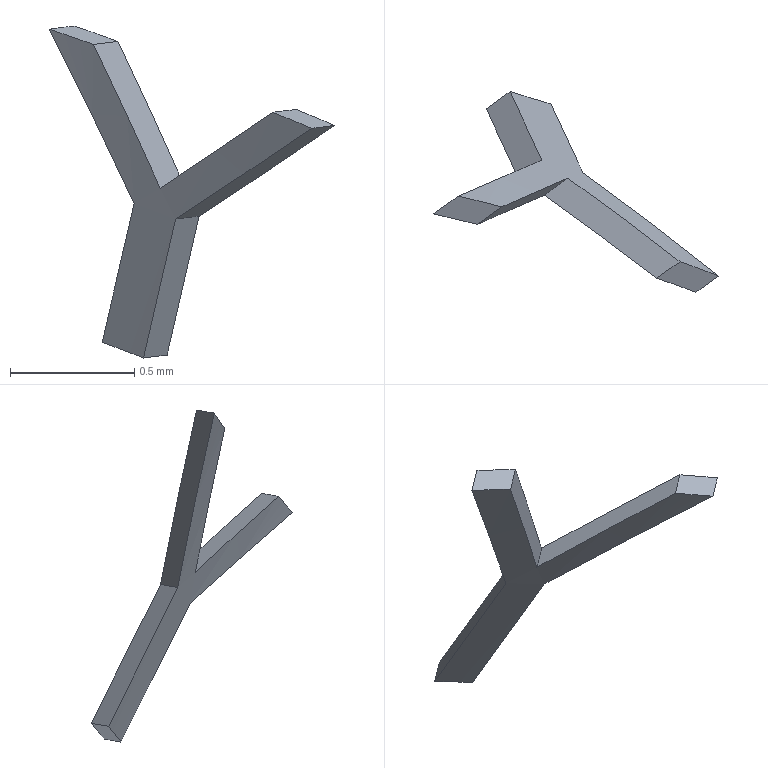Part | SolidWorks | features BaseBody 1 | 1 solid | 11 faces | box 1.15 x 0.8105 x 1.338 mm | volume 0.03304 mm3 | plane 9 | cylinder 2 | commonest cylinder face diameters 16.8 x1 17 x1
STEP:
#1=CARTESIAN_POINT('',(1969.96,-236.727,996.491));
#2=VERTEX_POINT('',#1);
#3=CARTESIAN_POINT('',(1970.089,-237.005,997.05));
#4=VERTEX_POINT('',#3);
#5=CARTESIAN_POINT('',(1970.77,-238.48,1000.016));
#6=DIRECTION('',(0.2015,-0.436,0.8771));
#7=VECTOR('',#6,1000.);
#8=LINE('',#5,#7);
#9=EDGE_CURVE('',#2,#4,#8,.T.);
#10=ORIENTED_EDGE('',*,*,#9,.T.);
#11=CARTESIAN_POINT('',(1970.638,-237.419,997.416));
#12=VERTEX_POINT('',#11);
#13=CARTESIAN_POINT('',(1970.089,-237.005,997.05));
#14=CARTESIAN_POINT('',(1970.275,-237.139,997.172));
#15=CARTESIAN_POINT('',(1970.458,-237.277,997.294));
#16=CARTESIAN_POINT('',(1970.638,-237.419,997.416));
#17=B_SPLINE_CURVE_WITH_KNOTS('',3,(#13,#14,#15,#16),.UNSPECIFIED.,.F.,.F.,(4,4),(0.,1.),.UNSPECIFIED.);
#18=EDGE_CURVE('',#4,#12,#17,.T.);
#19=ORIENTED_EDGE('',*,*,#18,.T.);
#20=CARTESIAN_POINT('',(1970.482,-237.362,997.481));
#21=VERTEX_POINT('',#20);
#22=CARTESIAN_POINT('',(1966.892,-244.458,994.777));
#23=DIRECTION('',(0.2015,-0.436,0.8771));
#24=DIRECTION('',(-0.7309,-0.6631,-0.1618));
#25=AXIS2_PLACEMENT_3D('',#22,#23,#24);
#26=CIRCLE('',#25,8.4);
#27=EDGE_CURVE('',#12,#21,#26,.T.);
#28=ORIENTED_EDGE('',*,*,#27,.T.);
#29=CARTESIAN_POINT('',(1970.027,-237.026,997.175));
#30=VERTEX_POINT('',#29);
#31=CARTESIAN_POINT('',(1970.027,-237.026,997.175));
#32=CARTESIAN_POINT('',(1970.181,-237.135,997.277));
#33=CARTESIAN_POINT('',(1970.332,-237.247,997.379));
#34=CARTESIAN_POINT('',(1970.482,-237.362,997.481));
#35=B_SPLINE_CURVE_WITH_KNOTS('',3,(#31,#32,#33,#34),.UNSPECIFIED.,.F.,.F.,(4,4),(0.,1.),.UNSPECIFIED.);
#36=EDGE_CURVE('',#30,#21,#35,.T.);
#37=ORIENTED_EDGE('',*,*,#36,.F.);
#38=CARTESIAN_POINT('',(1969.758,-237.145,997.754));
#39=VERTEX_POINT('',#38);
#40=CARTESIAN_POINT('',(1969.758,-237.145,997.754));
#41=CARTESIAN_POINT('',(1969.85,-237.104,997.563));
#42=CARTESIAN_POINT('',(1969.94,-237.064,997.37));
#43=CARTESIAN_POINT('',(1970.027,-237.026,997.175));
#44=B_SPLINE_CURVE_WITH_KNOTS('',3,(#40,#41,#42,#43),.UNSPECIFIED.,.F.,.F.,(4,4),(0.,1.),.UNSPECIFIED.);
#45=EDGE_CURVE('',#39,#30,#44,.T.);
#46=ORIENTED_EDGE('',*,*,#45,.F.);
#47=CARTESIAN_POINT('',(1969.58,-237.103,997.816));
#48=VERTEX_POINT('',#47);
#49=CARTESIAN_POINT('',(1966.892,-244.458,994.777));
#50=DIRECTION('',(0.2015,-0.436,0.8771));
#51=DIRECTION('',(-0.7309,-0.6631,-0.1618));
#52=AXIS2_PLACEMENT_3D('',#49,#50,#51);
#53=CIRCLE('',#52,8.4);
#54=EDGE_CURVE('',#39,#48,#53,.T.);
#55=ORIENTED_EDGE('',*,*,#54,.T.);
#56=CARTESIAN_POINT('',(1969.922,-236.955,997.114));
#57=VERTEX_POINT('',#56);
#58=CARTESIAN_POINT('',(1969.58,-237.103,997.816));
#59=CARTESIAN_POINT('',(1969.698,-237.051,997.585));
#60=CARTESIAN_POINT('',(1969.812,-237.002,997.35));
#61=CARTESIAN_POINT('',(1969.922,-236.955,997.114));
#62=B_SPLINE_CURVE_WITH_KNOTS('',3,(#58,#59,#60,#61),.UNSPECIFIED.,.F.,.F.,(4,4),(0.,1.),.UNSPECIFIED.);
#63=EDGE_CURVE('',#48,#57,#62,.T.);
#64=ORIENTED_EDGE('',*,*,#63,.T.);
#65=CARTESIAN_POINT('',(1969.793,-236.677,996.554));
#66=VERTEX_POINT('',#65);
#67=CARTESIAN_POINT('',(1970.603,-238.43,1000.08));
#68=DIRECTION('',(-0.2015,0.436,-0.8771));
#69=VECTOR('',#68,1000.);
#70=LINE('',#67,#69);
#71=EDGE_CURVE('',#57,#66,#70,.T.);
#72=ORIENTED_EDGE('',*,*,#71,.T.);
#73=CARTESIAN_POINT('',(1966.64,-243.913,993.681));
#74=DIRECTION('',(-0.2015,0.436,-0.8771));
#75=DIRECTION('',(-0.7309,-0.6631,-0.1618));
#76=AXIS2_PLACEMENT_3D('',#73,#74,#75);
#77=CIRCLE('',#76,8.4);
#78=EDGE_CURVE('',#66,#2,#77,.T.);
#79=ORIENTED_EDGE('',*,*,#78,.T.);
#80=EDGE_LOOP('',(#10,#19,#28,#37,#46,#55,#64,#72,#79));
#81=FACE_OUTER_BOUND('',#80,.T.);
#82=CARTESIAN_POINT('',(1967.45,-245.666,997.207));
#83=DIRECTION('',(0.2015,-0.436,0.8771));
#84=DIRECTION('',(-0.7309,-0.6631,-0.1618));
#85=AXIS2_PLACEMENT_3D('',#82,#83,#84);
#86=CYLINDRICAL_SURFACE('',#85,8.4);
#87=ADVANCED_FACE('',(#81),#86,.F.);
#88=CARTESIAN_POINT('',(1970.055,-236.659,996.503));
#89=VERTEX_POINT('',#88);
#90=CARTESIAN_POINT('',(1970.008,-236.693,996.497));
#91=DIRECTION('',(-0.8088,-0.5792,-0.1022));
#92=VECTOR('',#91,1000.);
#93=LINE('',#90,#92);
#94=EDGE_CURVE('',#89,#2,#93,.T.);
#95=ORIENTED_EDGE('',*,*,#94,.T.);
#96=ORIENTED_EDGE('',*,*,#78,.F.);
#97=CARTESIAN_POINT('',(1969.89,-236.608,996.566));
#98=VERTEX_POINT('',#97);
#99=CARTESIAN_POINT('',(1969.841,-236.643,996.56));
#100=DIRECTION('',(-0.8088,-0.5792,-0.1022));
#101=VECTOR('',#100,1000.);
#102=LINE('',#99,#101);
#103=EDGE_CURVE('',#98,#66,#102,.T.);
#104=ORIENTED_EDGE('',*,*,#103,.F.);
#105=CARTESIAN_POINT('',(1966.64,-243.913,993.681));
#106=DIRECTION('',(-0.2015,0.436,-0.8771));
#107=DIRECTION('',(-0.7309,-0.6631,-0.1618));
#108=AXIS2_PLACEMENT_3D('',#105,#106,#107);
#109=CIRCLE('',#108,8.5);
#110=EDGE_CURVE('',#98,#89,#109,.T.);
#111=ORIENTED_EDGE('',*,*,#110,.T.);
#112=EDGE_LOOP('',(#95,#96,#104,#111));
#113=FACE_OUTER_BOUND('',#112,.T.);
#114=CARTESIAN_POINT('',(1982.308,-239.633,992.21));
#115=DIRECTION('',(-0.2015,0.436,-0.8771));
#116=DIRECTION('',(-0.5526,0.6888,0.4693));
#117=AXIS2_PLACEMENT_3D('',#114,#115,#116);
#118=PLANE('',#117);
#119=ADVANCED_FACE('',(#113),#118,.T.);
#120=ORIENTED_EDGE('',*,*,#103,.T.);
#121=ORIENTED_EDGE('',*,*,#71,.F.);
#122=CARTESIAN_POINT('',(1970.018,-236.886,997.126));
#123=VERTEX_POINT('',#122);
#124=CARTESIAN_POINT('',(1969.97,-236.921,997.12));
#125=DIRECTION('',(-0.8088,-0.5792,-0.1022));
#126=VECTOR('',#125,1000.);
#127=LINE('',#124,#126);
#128=EDGE_CURVE('',#123,#57,#127,.T.);
#129=ORIENTED_EDGE('',*,*,#128,.F.);
#130=CARTESIAN_POINT('',(1969.954,-236.747,996.846));
#131=DIRECTION('',(-0.2015,0.436,-0.8771));
#132=VECTOR('',#131,1000.);
#133=LINE('',#130,#132);
#134=EDGE_CURVE('',#123,#98,#133,.T.);
#135=ORIENTED_EDGE('',*,*,#134,.T.);
#136=EDGE_LOOP('',(#120,#121,#129,#135));
#137=FACE_OUTER_BOUND('',#136,.T.);
#138=CARTESIAN_POINT('',(1976.364,-232.342,997.927));
#139=DIRECTION('',(-0.5526,0.6888,0.4693));
#140=DIRECTION('',(0.2015,-0.436,0.8771));
#141=AXIS2_PLACEMENT_3D('',#138,#139,#140);
#142=PLANE('',#141);
#143=ADVANCED_FACE('',(#137),#142,.T.);
#144=ORIENTED_EDGE('',*,*,#128,.T.);
#145=ORIENTED_EDGE('',*,*,#63,.F.);
#146=CARTESIAN_POINT('',(1969.681,-237.031,997.829));
#147=VERTEX_POINT('',#146);
#148=CARTESIAN_POINT('',(1969.63,-237.067,997.822));
#149=DIRECTION('',(-0.8088,-0.5792,-0.1022));
#150=VECTOR('',#149,1000.);
#151=LINE('',#148,#150);
#152=EDGE_CURVE('',#147,#48,#151,.T.);
#153=ORIENTED_EDGE('',*,*,#152,.F.);
#154=CARTESIAN_POINT('',(1969.681,-237.031,997.829));
#155=CARTESIAN_POINT('',(1969.751,-237.,997.69));
#156=CARTESIAN_POINT('',(1969.819,-236.971,997.55));
#157=CARTESIAN_POINT('',(1969.887,-236.942,997.409));
#158=CARTESIAN_POINT('',(1969.953,-236.914,997.268));
#159=CARTESIAN_POINT('',(1970.018,-236.886,997.126));
#160=B_SPLINE_CURVE_WITH_KNOTS('',5,(#154,#155,#156,#157,#158,#159),.UNSPECIFIED.,.F.,.F.,(6,6),(0.,1.),.UNSPECIFIED.);
#161=EDGE_CURVE('',#147,#123,#160,.T.);
#162=ORIENTED_EDGE('',*,*,#161,.T.);
#163=EDGE_LOOP('',(#144,#145,#153,#162));
#164=FACE_OUTER_BOUND('',#163,.T.);
#165=CARTESIAN_POINT('',(1976.257,-232.322,998.66));
#166=DIRECTION('',(-0.5701,0.8147,-0.1059));
#167=DIRECTION('',(-0.1446,0.02737,0.9891));
#168=AXIS2_PLACEMENT_3D('',#165,#166,#167);
#169=PLANE('',#168);
#170=ADVANCED_FACE('',(#164),#169,.T.);
#171=ORIENTED_EDGE('',*,*,#152,.T.);
#172=ORIENTED_EDGE('',*,*,#54,.F.);
#173=CARTESIAN_POINT('',(1969.857,-237.075,997.767));
#174=VERTEX_POINT('',#173);
#175=CARTESIAN_POINT('',(1969.807,-237.11,997.761));
#176=DIRECTION('',(-0.8088,-0.5792,-0.1022));
#177=VECTOR('',#176,1000.);
#178=LINE('',#175,#177);
#179=EDGE_CURVE('',#174,#39,#178,.T.);
#180=ORIENTED_EDGE('',*,*,#179,.F.);
#181=CARTESIAN_POINT('',(1966.892,-244.458,994.777));
#182=DIRECTION('',(0.2015,-0.436,0.8771));
#183=DIRECTION('',(-0.7309,-0.6631,-0.1618));
#184=AXIS2_PLACEMENT_3D('',#181,#182,#183);
#185=CIRCLE('',#184,8.5);
#186=EDGE_CURVE('',#174,#147,#185,.T.);
#187=ORIENTED_EDGE('',*,*,#186,.T.);
#188=EDGE_LOOP('',(#171,#172,#180,#187));
#189=FACE_OUTER_BOUND('',#188,.T.);
#190=CARTESIAN_POINT('',(1982.415,-239.999,993.428));
#191=DIRECTION('',(0.2015,-0.436,0.8771));
#192=DIRECTION('',(0.5526,-0.6888,-0.4693));
#193=AXIS2_PLACEMENT_3D('',#190,#191,#192);
#194=PLANE('',#193);
#195=ADVANCED_FACE('',(#189),#194,.T.);
#196=ORIENTED_EDGE('',*,*,#179,.T.);
#197=ORIENTED_EDGE('',*,*,#45,.T.);
#198=CARTESIAN_POINT('',(1970.123,-236.958,997.187));
#199=VERTEX_POINT('',#198);
#200=CARTESIAN_POINT('',(1970.075,-236.992,997.181));
#201=DIRECTION('',(-0.8088,-0.5792,-0.1022));
#202=VECTOR('',#201,1000.);
#203=LINE('',#200,#202);
#204=EDGE_CURVE('',#199,#30,#203,.T.);
#205=ORIENTED_EDGE('',*,*,#204,.F.);
#206=CARTESIAN_POINT('',(1969.857,-237.075,997.767));
#207=CARTESIAN_POINT('',(1969.912,-237.05,997.652));
#208=CARTESIAN_POINT('',(1969.966,-237.026,997.536));
#209=CARTESIAN_POINT('',(1970.019,-237.003,997.421));
#210=CARTESIAN_POINT('',(1970.071,-236.98,997.304));
#211=CARTESIAN_POINT('',(1970.123,-236.958,997.187));
#212=B_SPLINE_CURVE_WITH_KNOTS('',5,(#206,#207,#208,#209,#210,#211),.UNSPECIFIED.,.F.,.F.,(6,6),(0.,1.),.UNSPECIFIED.);
#213=EDGE_CURVE('',#174,#199,#212,.T.);
#214=ORIENTED_EDGE('',*,*,#213,.F.);
#215=EDGE_LOOP('',(#196,#197,#205,#214));
#216=FACE_OUTER_BOUND('',#215,.T.);
#217=CARTESIAN_POINT('',(1976.428,-232.442,997.984));
#218=DIRECTION('',(0.5712,-0.8149,0.09826));
#219=DIRECTION('',(0.1402,-0.0211,-0.9899));
#220=AXIS2_PLACEMENT_3D('',#217,#218,#219);
#221=PLANE('',#220);
#222=ADVANCED_FACE('',(#216),#221,.T.);
#223=ORIENTED_EDGE('',*,*,#204,.T.);
#224=ORIENTED_EDGE('',*,*,#36,.T.);
#225=CARTESIAN_POINT('',(1970.575,-237.295,997.492));
#226=VERTEX_POINT('',#225);
#227=CARTESIAN_POINT('',(1970.528,-237.328,997.486));
#228=DIRECTION('',(-0.8088,-0.5792,-0.1022));
#229=VECTOR('',#228,1000.);
#230=LINE('',#227,#229);
#231=EDGE_CURVE('',#226,#21,#230,.T.);
#232=ORIENTED_EDGE('',*,*,#231,.F.);
#233=CARTESIAN_POINT('',(1970.123,-236.958,997.187));
#234=CARTESIAN_POINT('',(1970.214,-237.024,997.248));
#235=CARTESIAN_POINT('',(1970.305,-237.09,997.309));
#236=CARTESIAN_POINT('',(1970.396,-237.158,997.37));
#237=CARTESIAN_POINT('',(1970.485,-237.226,997.431));
#238=CARTESIAN_POINT('',(1970.575,-237.295,997.492));
#239=B_SPLINE_CURVE_WITH_KNOTS('',5,(#233,#234,#235,#236,#237,#238),.UNSPECIFIED.,.F.,.F.,(6,6),(0.,1.),.UNSPECIFIED.);
#240=EDGE_CURVE('',#199,#226,#239,.T.);
#241=ORIENTED_EDGE('',*,*,#240,.F.);
#242=EDGE_LOOP('',(#223,#224,#232,#241));
#243=FACE_OUTER_BOUND('',#242,.T.);
#244=CARTESIAN_POINT('',(1976.717,-232.896,998.268));
#245=DIRECTION('',(-0.3469,0.3295,0.8781));
#246=DIRECTION('',(0.4749,-0.7456,0.4674));
#247=AXIS2_PLACEMENT_3D('',#244,#245,#246);
#248=PLANE('',#247);
#249=ADVANCED_FACE('',(#243),#248,.T.);
#250=ORIENTED_EDGE('',*,*,#231,.T.);
#251=ORIENTED_EDGE('',*,*,#27,.F.);
#252=CARTESIAN_POINT('',(1970.73,-237.353,997.428));
#253=VERTEX_POINT('',#252);
#254=CARTESIAN_POINT('',(1970.684,-237.386,997.422));
#255=DIRECTION('',(-0.8088,-0.5792,-0.1022));
#256=VECTOR('',#255,1000.);
#257=LINE('',#254,#256);
#258=EDGE_CURVE('',#253,#12,#257,.T.);
#259=ORIENTED_EDGE('',*,*,#258,.F.);
#260=CARTESIAN_POINT('',(1966.892,-244.458,994.777));
#261=DIRECTION('',(0.2015,-0.436,0.8771));
#262=DIRECTION('',(-0.7309,-0.6631,-0.1618));
#263=AXIS2_PLACEMENT_3D('',#260,#261,#262);
#264=CIRCLE('',#263,8.5);
#265=EDGE_CURVE('',#253,#226,#264,.T.);
#266=ORIENTED_EDGE('',*,*,#265,.T.);
#267=EDGE_LOOP('',(#250,#251,#259,#266));
#268=FACE_OUTER_BOUND('',#267,.T.);
#269=CARTESIAN_POINT('',(1982.415,-239.999,993.428));
#270=DIRECTION('',(0.2015,-0.436,0.8771));
#271=DIRECTION('',(0.5526,-0.6888,-0.4693));
#272=AXIS2_PLACEMENT_3D('',#269,#270,#271);
#273=PLANE('',#272);
#274=ADVANCED_FACE('',(#268),#273,.T.);
#275=ORIENTED_EDGE('',*,*,#258,.T.);
#276=ORIENTED_EDGE('',*,*,#18,.F.);
#277=CARTESIAN_POINT('',(1970.184,-236.937,997.062));
#278=VERTEX_POINT('',#277);
#279=CARTESIAN_POINT('',(1970.136,-236.971,997.056));
#280=DIRECTION('',(-0.8088,-0.5792,-0.1022));
#281=VECTOR('',#280,1000.);
#282=LINE('',#279,#281);
#283=EDGE_CURVE('',#278,#4,#282,.T.);
#284=ORIENTED_EDGE('',*,*,#283,.F.);
#285=CARTESIAN_POINT('',(1970.184,-236.937,997.062));
#286=CARTESIAN_POINT('',(1970.295,-237.018,997.135));
#287=CARTESIAN_POINT('',(1970.405,-237.1,997.208));
#288=CARTESIAN_POINT('',(1970.514,-237.183,997.281));
#289=CARTESIAN_POINT('',(1970.623,-237.267,997.355));
#290=CARTESIAN_POINT('',(1970.73,-237.353,997.428));
#291=B_SPLINE_CURVE_WITH_KNOTS('',5,(#285,#286,#287,#288,#289,#290),.UNSPECIFIED.,.F.,.F.,(6,6),(0.,1.),.UNSPECIFIED.);
#292=EDGE_CURVE('',#278,#253,#291,.T.);
#293=ORIENTED_EDGE('',*,*,#292,.T.);
#294=EDGE_LOOP('',(#275,#276,#284,#293));
#295=FACE_OUTER_BOUND('',#294,.T.);
#296=CARTESIAN_POINT('',(1976.45,-232.45,997.854));
#297=DIRECTION('',(0.3433,-0.3238,-0.8817));
#298=DIRECTION('',(-0.4776,0.7481,-0.4607));
#299=AXIS2_PLACEMENT_3D('',#296,#297,#298);
#300=PLANE('',#299);
#301=ADVANCED_FACE('',(#295),#300,.T.);
#302=ORIENTED_EDGE('',*,*,#283,.T.);
#303=ORIENTED_EDGE('',*,*,#9,.F.);
#304=ORIENTED_EDGE('',*,*,#94,.F.);
#305=CARTESIAN_POINT('',(1970.119,-236.798,996.783));
#306=DIRECTION('',(0.2015,-0.436,0.8771));
#307=VECTOR('',#306,1000.);
#308=LINE('',#305,#307);
#309=EDGE_CURVE('',#89,#278,#308,.T.);
#310=ORIENTED_EDGE('',*,*,#309,.T.);
#311=EDGE_LOOP('',(#302,#303,#304,#310));
#312=FACE_OUTER_BOUND('',#311,.T.);
#313=CARTESIAN_POINT('',(1976.321,-232.171,997.294));
#314=DIRECTION('',(0.5526,-0.6888,-0.4693));
#315=DIRECTION('',(-0.2015,0.436,-0.8771));
#316=AXIS2_PLACEMENT_3D('',#313,#314,#315);
#317=PLANE('',#316);
#318=ADVANCED_FACE('',(#312),#317,.T.);
#319=ORIENTED_EDGE('',*,*,#110,.F.);
#320=ORIENTED_EDGE('',*,*,#134,.F.);
#321=ORIENTED_EDGE('',*,*,#161,.F.);
#322=ORIENTED_EDGE('',*,*,#186,.F.);
#323=ORIENTED_EDGE('',*,*,#213,.T.);
#324=ORIENTED_EDGE('',*,*,#240,.T.);
#325=ORIENTED_EDGE('',*,*,#265,.F.);
#326=ORIENTED_EDGE('',*,*,#292,.F.);
#327=ORIENTED_EDGE('',*,*,#309,.F.);
#328=EDGE_LOOP('',(#319,#320,#321,#322,#323,#324,#325,#326,#327));
#329=FACE_OUTER_BOUND('',#328,.T.);
#330=CARTESIAN_POINT('',(1967.45,-245.666,997.207));
#331=DIRECTION('',(0.2015,-0.436,0.8771));
#332=DIRECTION('',(-0.7309,-0.6631,-0.1618));
#333=AXIS2_PLACEMENT_3D('',#330,#331,#332);
#334=CYLINDRICAL_SURFACE('',#333,8.5);
#335=ADVANCED_FACE('',(#329),#334,.T.);
#336=CLOSED_SHELL('',(#87,#119,#143,#170,#195,#222,#249,#274,#301,#318,#335));
#337=MANIFOLD_SOLID_BREP('',#336);
#338=CARTESIAN_POINT('',(0.,0.,0.));
#339=DIRECTION('',(0.,0.,1.));
#340=DIRECTION('',(1.,0.,0.));
#341=AXIS2_PLACEMENT_3D('',#338,#339,#340);
#342=(LENGTH_UNIT()NAMED_UNIT(*)SI_UNIT(.MILLI.,.METRE.));
#343=UNCERTAINTY_MEASURE_WITH_UNIT(LENGTH_MEASURE(0.00001),#342,'','');
#344=(NAMED_UNIT(*)PLANE_ANGLE_UNIT()SI_UNIT($,.RADIAN.));
#345=(NAMED_UNIT(*)SI_UNIT($,.STERADIAN.)SOLID_ANGLE_UNIT());
#346=(GEOMETRIC_REPRESENTATION_CONTEXT(3)GLOBAL_UNCERTAINTY_ASSIGNED_CONTEXT((#343))GLOBAL_UNIT_ASSIGNED_CONTEXT((#342,#344,#345))REPRESENTATION_CONTEXT('',''));
#347=ADVANCED_BREP_SHAPE_REPRESENTATION('',(#337,#341),#346);